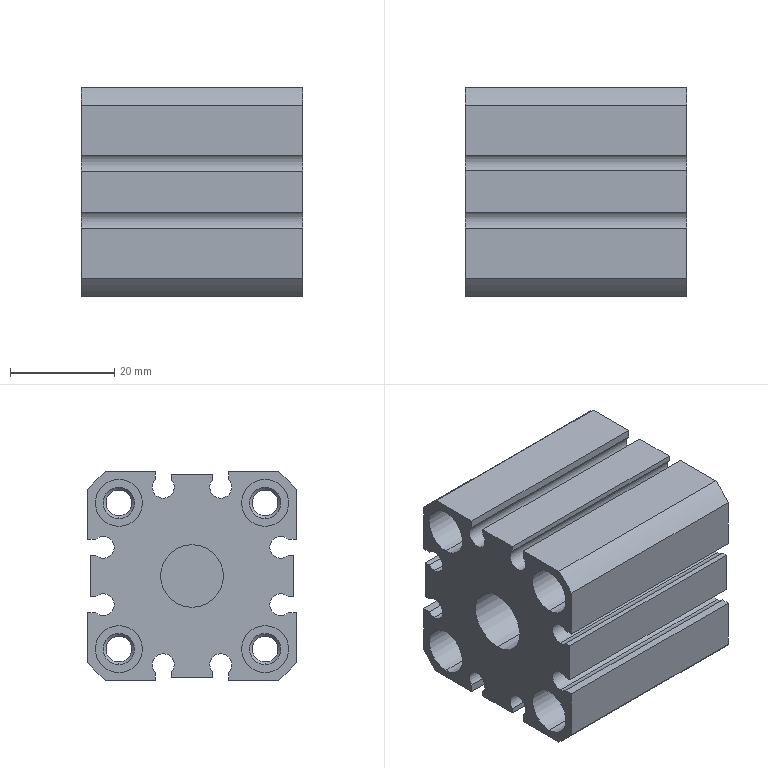Part | SolidWorks | features RefAxis 18, 3DProfileFeature 6, HoleWzd 2, RevCut 2, Extrusion 1, LPattern 1 | 1 solid | 150 faces | box 42.5 x 40 x 40 mm | volume 45351 mm3 | cylinder 70 | cone 40 | plane 40 | commonest cylinder face diameters 4.2 x18 4.917 x16 9 x16 5.4 x8 4.134 x4 52 x4